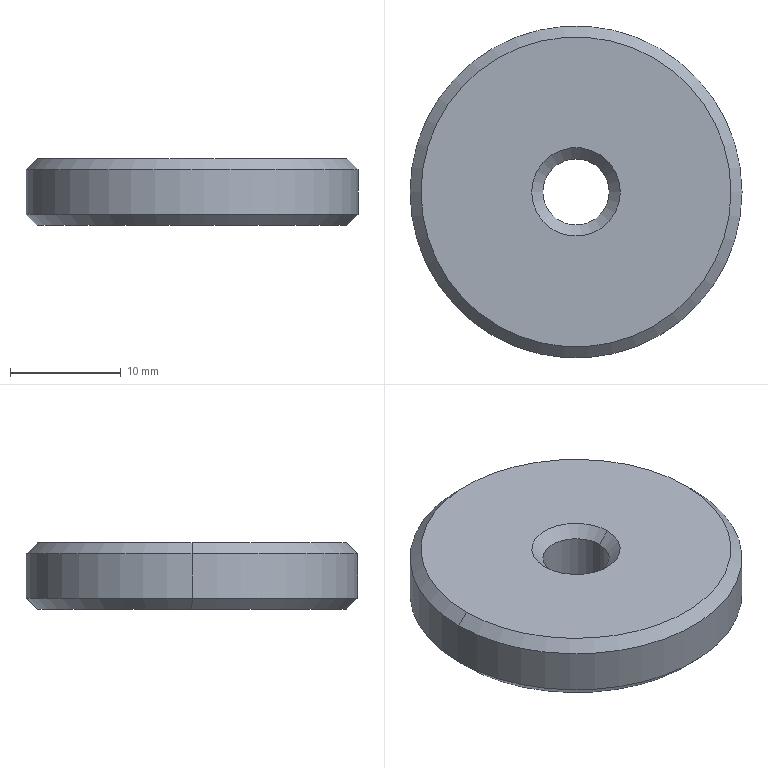Part | STEP file | Pressure plate | 1 solid | 14 faces | box 30 x 30 x 6 mm | volume 3958 mm3 | cone 8 | cylinder 4 | plane 2 | commonest cylinder face diameters 6 x2 30 x2
STEP:
#1=CARTESIAN_POINT('',(14.,0.,0.));
#2=VERTEX_POINT('',#1);
#3=CARTESIAN_POINT('',(-14.,0.,0.));
#4=VERTEX_POINT('',#3);
#5=CARTESIAN_POINT('',(0.,0.,0.));
#6=DIRECTION('',(0.,0.,1.));
#7=DIRECTION('',(1.,0.,0.));
#8=AXIS2_PLACEMENT_3D('',#5,#6,#7);
#9=CIRCLE('',#8,14.);
#10=EDGE_CURVE('',#2,#4,#9,.T.);
#11=ORIENTED_EDGE('',*,*,#10,.T.);
#12=CARTESIAN_POINT('',(-15.,0.,1.));
#13=VERTEX_POINT('',#12);
#14=CARTESIAN_POINT('',(-15.,0.,1.));
#15=DIRECTION('',(-0.7071,0.,0.7071));
#16=VECTOR('',#15,1000.);
#17=LINE('',#14,#16);
#18=EDGE_CURVE('',#4,#13,#17,.T.);
#19=ORIENTED_EDGE('',*,*,#18,.T.);
#20=CARTESIAN_POINT('',(15.,0.,1.));
#21=VERTEX_POINT('',#20);
#22=CARTESIAN_POINT('',(0.,0.,1.));
#23=DIRECTION('',(0.,0.,-1.));
#24=DIRECTION('',(1.,0.,0.));
#25=AXIS2_PLACEMENT_3D('',#22,#23,#24);
#26=CIRCLE('',#25,15.);
#27=EDGE_CURVE('',#13,#21,#26,.T.);
#28=ORIENTED_EDGE('',*,*,#27,.T.);
#29=CARTESIAN_POINT('',(15.,0.,1.));
#30=DIRECTION('',(0.7071,0.,0.7071));
#31=VECTOR('',#30,1000.);
#32=LINE('',#29,#31);
#33=EDGE_CURVE('',#2,#21,#32,.T.);
#34=ORIENTED_EDGE('',*,*,#33,.F.);
#35=EDGE_LOOP('',(#11,#19,#28,#34));
#36=FACE_OUTER_BOUND('',#35,.T.);
#37=CARTESIAN_POINT('',(0.,0.,1.));
#38=DIRECTION('',(0.,0.,1.));
#39=DIRECTION('',(1.,0.,0.));
#40=AXIS2_PLACEMENT_3D('',#37,#38,#39);
#41=CONICAL_SURFACE('',#40,15.,0.7854);
#42=ADVANCED_FACE('',(#36),#41,.T.);
#43=CARTESIAN_POINT('',(3.,0.,1.));
#44=VERTEX_POINT('',#43);
#45=CARTESIAN_POINT('',(-3.,0.,1.));
#46=VERTEX_POINT('',#45);
#47=CARTESIAN_POINT('',(0.,0.,1.));
#48=DIRECTION('',(0.,0.,-1.));
#49=DIRECTION('',(-1.,0.,0.));
#50=AXIS2_PLACEMENT_3D('',#47,#48,#49);
#51=CIRCLE('',#50,3.);
#52=EDGE_CURVE('',#44,#46,#51,.T.);
#53=ORIENTED_EDGE('',*,*,#52,.F.);
#54=CARTESIAN_POINT('',(4.,0.,0.));
#55=VERTEX_POINT('',#54);
#56=CARTESIAN_POINT('',(4.,0.,0.));
#57=DIRECTION('',(0.7071,0.,-0.7071));
#58=VECTOR('',#57,1000.);
#59=LINE('',#56,#58);
#60=EDGE_CURVE('',#44,#55,#59,.T.);
#61=ORIENTED_EDGE('',*,*,#60,.T.);
#62=CARTESIAN_POINT('',(-4.,0.,0.));
#63=VERTEX_POINT('',#62);
#64=CARTESIAN_POINT('',(0.,0.,0.));
#65=DIRECTION('',(0.,0.,-1.));
#66=DIRECTION('',(-1.,0.,0.));
#67=AXIS2_PLACEMENT_3D('',#64,#65,#66);
#68=CIRCLE('',#67,4.);
#69=EDGE_CURVE('',#55,#63,#68,.T.);
#70=ORIENTED_EDGE('',*,*,#69,.T.);
#71=CARTESIAN_POINT('',(-4.,0.,0.));
#72=DIRECTION('',(-0.7071,0.,-0.7071));
#73=VECTOR('',#72,1000.);
#74=LINE('',#71,#73);
#75=EDGE_CURVE('',#46,#63,#74,.T.);
#76=ORIENTED_EDGE('',*,*,#75,.F.);
#77=EDGE_LOOP('',(#53,#61,#70,#76));
#78=FACE_OUTER_BOUND('',#77,.T.);
#79=CARTESIAN_POINT('',(0.,0.,0.));
#80=DIRECTION('',(0.,0.,-1.));
#81=DIRECTION('',(-1.,0.,0.));
#82=AXIS2_PLACEMENT_3D('',#79,#80,#81);
#83=CONICAL_SURFACE('',#82,4.,0.7854);
#84=ADVANCED_FACE('',(#78),#83,.F.);
#85=CARTESIAN_POINT('',(-15.,0.,5.));
#86=VERTEX_POINT('',#85);
#87=CARTESIAN_POINT('',(15.,0.,5.));
#88=VERTEX_POINT('',#87);
#89=CARTESIAN_POINT('',(0.,0.,5.));
#90=DIRECTION('',(0.,0.,-1.));
#91=DIRECTION('',(-1.,0.,0.));
#92=AXIS2_PLACEMENT_3D('',#89,#90,#91);
#93=CIRCLE('',#92,15.);
#94=EDGE_CURVE('',#86,#88,#93,.T.);
#95=ORIENTED_EDGE('',*,*,#94,.T.);
#96=CARTESIAN_POINT('',(15.,0.,6.));
#97=DIRECTION('',(0.,0.,-1.));
#98=VECTOR('',#97,1000.);
#99=LINE('',#96,#98);
#100=EDGE_CURVE('',#88,#21,#99,.T.);
#101=ORIENTED_EDGE('',*,*,#100,.T.);
#102=ORIENTED_EDGE('',*,*,#27,.F.);
#103=CARTESIAN_POINT('',(-15.,0.,6.));
#104=DIRECTION('',(0.,0.,-1.));
#105=VECTOR('',#104,1000.);
#106=LINE('',#103,#105);
#107=EDGE_CURVE('',#86,#13,#106,.T.);
#108=ORIENTED_EDGE('',*,*,#107,.F.);
#109=EDGE_LOOP('',(#95,#101,#102,#108));
#110=FACE_OUTER_BOUND('',#109,.T.);
#111=CARTESIAN_POINT('',(0.,0.,6.));
#112=DIRECTION('',(0.,0.,-1.));
#113=DIRECTION('',(-1.,0.,0.));
#114=AXIS2_PLACEMENT_3D('',#111,#112,#113);
#115=CYLINDRICAL_SURFACE('',#114,15.);
#116=ADVANCED_FACE('',(#110),#115,.T.);
#117=CARTESIAN_POINT('',(3.,0.,5.));
#118=VERTEX_POINT('',#117);
#119=CARTESIAN_POINT('',(-3.,0.,5.));
#120=VERTEX_POINT('',#119);
#121=CARTESIAN_POINT('',(0.,0.,5.));
#122=DIRECTION('',(0.,0.,-1.));
#123=DIRECTION('',(-1.,0.,0.));
#124=AXIS2_PLACEMENT_3D('',#121,#122,#123);
#125=CIRCLE('',#124,3.);
#126=EDGE_CURVE('',#118,#120,#125,.T.);
#127=ORIENTED_EDGE('',*,*,#126,.F.);
#128=CARTESIAN_POINT('',(3.,0.,6.));
#129=DIRECTION('',(0.,0.,-1.));
#130=VECTOR('',#129,1000.);
#131=LINE('',#128,#130);
#132=EDGE_CURVE('',#118,#44,#131,.T.);
#133=ORIENTED_EDGE('',*,*,#132,.T.);
#134=ORIENTED_EDGE('',*,*,#52,.T.);
#135=CARTESIAN_POINT('',(-3.,0.,6.));
#136=DIRECTION('',(0.,0.,-1.));
#137=VECTOR('',#136,1000.);
#138=LINE('',#135,#137);
#139=EDGE_CURVE('',#120,#46,#138,.T.);
#140=ORIENTED_EDGE('',*,*,#139,.F.);
#141=EDGE_LOOP('',(#127,#133,#134,#140));
#142=FACE_OUTER_BOUND('',#141,.T.);
#143=CARTESIAN_POINT('',(0.,0.,6.));
#144=DIRECTION('',(0.,0.,-1.));
#145=DIRECTION('',(-1.,0.,0.));
#146=AXIS2_PLACEMENT_3D('',#143,#144,#145);
#147=CYLINDRICAL_SURFACE('',#146,3.);
#148=ADVANCED_FACE('',(#142),#147,.F.);
#149=CARTESIAN_POINT('',(-14.,0.,6.));
#150=VERTEX_POINT('',#149);
#151=CARTESIAN_POINT('',(14.,0.,6.));
#152=VERTEX_POINT('',#151);
#153=CARTESIAN_POINT('',(0.,0.,6.));
#154=DIRECTION('',(0.,0.,-1.));
#155=DIRECTION('',(-1.,0.,0.));
#156=AXIS2_PLACEMENT_3D('',#153,#154,#155);
#157=CIRCLE('',#156,14.);
#158=EDGE_CURVE('',#150,#152,#157,.T.);
#159=ORIENTED_EDGE('',*,*,#158,.T.);
#160=CARTESIAN_POINT('',(15.,0.,5.));
#161=DIRECTION('',(0.7071,0.,-0.7071));
#162=VECTOR('',#161,1000.);
#163=LINE('',#160,#162);
#164=EDGE_CURVE('',#152,#88,#163,.T.);
#165=ORIENTED_EDGE('',*,*,#164,.T.);
#166=ORIENTED_EDGE('',*,*,#94,.F.);
#167=CARTESIAN_POINT('',(-15.,0.,5.));
#168=DIRECTION('',(-0.7071,0.,-0.7071));
#169=VECTOR('',#168,1000.);
#170=LINE('',#167,#169);
#171=EDGE_CURVE('',#150,#86,#170,.T.);
#172=ORIENTED_EDGE('',*,*,#171,.F.);
#173=EDGE_LOOP('',(#159,#165,#166,#172));
#174=FACE_OUTER_BOUND('',#173,.T.);
#175=CARTESIAN_POINT('',(0.,0.,5.));
#176=DIRECTION('',(0.,0.,-1.));
#177=DIRECTION('',(-1.,0.,0.));
#178=AXIS2_PLACEMENT_3D('',#175,#176,#177);
#179=CONICAL_SURFACE('',#178,15.,0.7854);
#180=ADVANCED_FACE('',(#174),#179,.T.);
#181=ORIENTED_EDGE('',*,*,#126,.T.);
#182=CARTESIAN_POINT('',(-4.,0.,6.));
#183=VERTEX_POINT('',#182);
#184=CARTESIAN_POINT('',(-4.,0.,6.));
#185=DIRECTION('',(-0.7071,0.,0.7071));
#186=VECTOR('',#185,1000.);
#187=LINE('',#184,#186);
#188=EDGE_CURVE('',#120,#183,#187,.T.);
#189=ORIENTED_EDGE('',*,*,#188,.T.);
#190=CARTESIAN_POINT('',(4.,0.,6.));
#191=VERTEX_POINT('',#190);
#192=CARTESIAN_POINT('',(0.,0.,6.));
#193=DIRECTION('',(0.,0.,-1.));
#194=DIRECTION('',(1.,0.,0.));
#195=AXIS2_PLACEMENT_3D('',#192,#193,#194);
#196=CIRCLE('',#195,4.);
#197=EDGE_CURVE('',#191,#183,#196,.T.);
#198=ORIENTED_EDGE('',*,*,#197,.F.);
#199=CARTESIAN_POINT('',(4.,0.,6.));
#200=DIRECTION('',(0.7071,0.,0.7071));
#201=VECTOR('',#200,1000.);
#202=LINE('',#199,#201);
#203=EDGE_CURVE('',#118,#191,#202,.T.);
#204=ORIENTED_EDGE('',*,*,#203,.F.);
#205=EDGE_LOOP('',(#181,#189,#198,#204));
#206=FACE_OUTER_BOUND('',#205,.T.);
#207=CARTESIAN_POINT('',(0.,0.,6.));
#208=DIRECTION('',(0.,0.,1.));
#209=DIRECTION('',(1.,0.,0.));
#210=AXIS2_PLACEMENT_3D('',#207,#208,#209);
#211=CONICAL_SURFACE('',#210,4.,0.7854);
#212=ADVANCED_FACE('',(#206),#211,.F.);
#213=ORIENTED_EDGE('',*,*,#10,.F.);
#214=CARTESIAN_POINT('',(0.,0.,0.));
#215=DIRECTION('',(0.,0.,1.));
#216=DIRECTION('',(1.,0.,0.));
#217=AXIS2_PLACEMENT_3D('',#214,#215,#216);
#218=CIRCLE('',#217,14.);
#219=EDGE_CURVE('',#4,#2,#218,.T.);
#220=ORIENTED_EDGE('',*,*,#219,.F.);
#221=EDGE_LOOP('',(#213,#220));
#222=FACE_OUTER_BOUND('',#221,.T.);
#223=CARTESIAN_POINT('',(0.,0.,0.));
#224=DIRECTION('',(0.,0.,-1.));
#225=DIRECTION('',(-1.,0.,0.));
#226=AXIS2_PLACEMENT_3D('',#223,#224,#225);
#227=CIRCLE('',#226,4.);
#228=EDGE_CURVE('',#63,#55,#227,.T.);
#229=ORIENTED_EDGE('',*,*,#228,.F.);
#230=ORIENTED_EDGE('',*,*,#69,.F.);
#231=EDGE_LOOP('',(#229,#230));
#232=FACE_BOUND('',#231,.T.);
#233=CARTESIAN_POINT('',(0.,0.,0.));
#234=DIRECTION('',(0.,0.,1.));
#235=DIRECTION('',(1.,0.,0.));
#236=AXIS2_PLACEMENT_3D('',#233,#234,#235);
#237=PLANE('',#236);
#238=ADVANCED_FACE('',(#222,#232),#237,.F.);
#239=ORIENTED_EDGE('',*,*,#18,.F.);
#240=ORIENTED_EDGE('',*,*,#219,.T.);
#241=ORIENTED_EDGE('',*,*,#33,.T.);
#242=CARTESIAN_POINT('',(0.,0.,1.));
#243=DIRECTION('',(0.,0.,-1.));
#244=DIRECTION('',(1.,0.,0.));
#245=AXIS2_PLACEMENT_3D('',#242,#243,#244);
#246=CIRCLE('',#245,15.);
#247=EDGE_CURVE('',#21,#13,#246,.T.);
#248=ORIENTED_EDGE('',*,*,#247,.T.);
#249=EDGE_LOOP('',(#239,#240,#241,#248));
#250=FACE_OUTER_BOUND('',#249,.T.);
#251=CARTESIAN_POINT('',(0.,0.,1.));
#252=DIRECTION('',(0.,0.,1.));
#253=DIRECTION('',(1.,0.,0.));
#254=AXIS2_PLACEMENT_3D('',#251,#252,#253);
#255=CONICAL_SURFACE('',#254,15.,0.7854);
#256=ADVANCED_FACE('',(#250),#255,.T.);
#257=ORIENTED_EDGE('',*,*,#60,.F.);
#258=CARTESIAN_POINT('',(0.,0.,1.));
#259=DIRECTION('',(0.,0.,-1.));
#260=DIRECTION('',(-1.,0.,0.));
#261=AXIS2_PLACEMENT_3D('',#258,#259,#260);
#262=CIRCLE('',#261,3.);
#263=EDGE_CURVE('',#46,#44,#262,.T.);
#264=ORIENTED_EDGE('',*,*,#263,.F.);
#265=ORIENTED_EDGE('',*,*,#75,.T.);
#266=ORIENTED_EDGE('',*,*,#228,.T.);
#267=EDGE_LOOP('',(#257,#264,#265,#266));
#268=FACE_OUTER_BOUND('',#267,.T.);
#269=CARTESIAN_POINT('',(0.,0.,0.));
#270=DIRECTION('',(0.,0.,-1.));
#271=DIRECTION('',(-1.,0.,0.));
#272=AXIS2_PLACEMENT_3D('',#269,#270,#271);
#273=CONICAL_SURFACE('',#272,4.,0.7854);
#274=ADVANCED_FACE('',(#268),#273,.F.);
#275=ORIENTED_EDGE('',*,*,#100,.F.);
#276=CARTESIAN_POINT('',(0.,0.,5.));
#277=DIRECTION('',(0.,0.,-1.));
#278=DIRECTION('',(-1.,0.,0.));
#279=AXIS2_PLACEMENT_3D('',#276,#277,#278);
#280=CIRCLE('',#279,15.);
#281=EDGE_CURVE('',#88,#86,#280,.T.);
#282=ORIENTED_EDGE('',*,*,#281,.T.);
#283=ORIENTED_EDGE('',*,*,#107,.T.);
#284=ORIENTED_EDGE('',*,*,#247,.F.);
#285=EDGE_LOOP('',(#275,#282,#283,#284));
#286=FACE_OUTER_BOUND('',#285,.T.);
#287=CARTESIAN_POINT('',(0.,0.,6.));
#288=DIRECTION('',(0.,0.,-1.));
#289=DIRECTION('',(-1.,0.,0.));
#290=AXIS2_PLACEMENT_3D('',#287,#288,#289);
#291=CYLINDRICAL_SURFACE('',#290,15.);
#292=ADVANCED_FACE('',(#286),#291,.T.);
#293=ORIENTED_EDGE('',*,*,#132,.F.);
#294=CARTESIAN_POINT('',(0.,0.,5.));
#295=DIRECTION('',(0.,0.,-1.));
#296=DIRECTION('',(-1.,0.,0.));
#297=AXIS2_PLACEMENT_3D('',#294,#295,#296);
#298=CIRCLE('',#297,3.);
#299=EDGE_CURVE('',#120,#118,#298,.T.);
#300=ORIENTED_EDGE('',*,*,#299,.F.);
#301=ORIENTED_EDGE('',*,*,#139,.T.);
#302=ORIENTED_EDGE('',*,*,#263,.T.);
#303=EDGE_LOOP('',(#293,#300,#301,#302));
#304=FACE_OUTER_BOUND('',#303,.T.);
#305=CARTESIAN_POINT('',(0.,0.,6.));
#306=DIRECTION('',(0.,0.,-1.));
#307=DIRECTION('',(-1.,0.,0.));
#308=AXIS2_PLACEMENT_3D('',#305,#306,#307);
#309=CYLINDRICAL_SURFACE('',#308,3.);
#310=ADVANCED_FACE('',(#304),#309,.F.);
#311=ORIENTED_EDGE('',*,*,#164,.F.);
#312=CARTESIAN_POINT('',(0.,0.,6.));
#313=DIRECTION('',(0.,0.,-1.));
#314=DIRECTION('',(-1.,0.,0.));
#315=AXIS2_PLACEMENT_3D('',#312,#313,#314);
#316=CIRCLE('',#315,14.);
#317=EDGE_CURVE('',#152,#150,#316,.T.);
#318=ORIENTED_EDGE('',*,*,#317,.T.);
#319=ORIENTED_EDGE('',*,*,#171,.T.);
#320=ORIENTED_EDGE('',*,*,#281,.F.);
#321=EDGE_LOOP('',(#311,#318,#319,#320));
#322=FACE_OUTER_BOUND('',#321,.T.);
#323=CARTESIAN_POINT('',(0.,0.,5.));
#324=DIRECTION('',(0.,0.,-1.));
#325=DIRECTION('',(-1.,0.,0.));
#326=AXIS2_PLACEMENT_3D('',#323,#324,#325);
#327=CONICAL_SURFACE('',#326,15.,0.7854);
#328=ADVANCED_FACE('',(#322),#327,.T.);
#329=ORIENTED_EDGE('',*,*,#188,.F.);
#330=ORIENTED_EDGE('',*,*,#299,.T.);
#331=ORIENTED_EDGE('',*,*,#203,.T.);
#332=CARTESIAN_POINT('',(0.,0.,6.));
#333=DIRECTION('',(0.,0.,-1.));
#334=DIRECTION('',(1.,0.,0.));
#335=AXIS2_PLACEMENT_3D('',#332,#333,#334);
#336=CIRCLE('',#335,4.);
#337=EDGE_CURVE('',#183,#191,#336,.T.);
#338=ORIENTED_EDGE('',*,*,#337,.F.);
#339=EDGE_LOOP('',(#329,#330,#331,#338));
#340=FACE_OUTER_BOUND('',#339,.T.);
#341=CARTESIAN_POINT('',(0.,0.,6.));
#342=DIRECTION('',(0.,0.,1.));
#343=DIRECTION('',(1.,0.,0.));
#344=AXIS2_PLACEMENT_3D('',#341,#342,#343);
#345=CONICAL_SURFACE('',#344,4.,0.7854);
#346=ADVANCED_FACE('',(#340),#345,.F.);
#347=ORIENTED_EDGE('',*,*,#158,.F.);
#348=ORIENTED_EDGE('',*,*,#317,.F.);
#349=EDGE_LOOP('',(#347,#348));
#350=FACE_OUTER_BOUND('',#349,.T.);
#351=ORIENTED_EDGE('',*,*,#197,.T.);
#352=ORIENTED_EDGE('',*,*,#337,.T.);
#353=EDGE_LOOP('',(#351,#352));
#354=FACE_BOUND('',#353,.T.);
#355=CARTESIAN_POINT('',(0.,0.,6.));
#356=DIRECTION('',(0.,0.,1.));
#357=DIRECTION('',(1.,0.,0.));
#358=AXIS2_PLACEMENT_3D('',#355,#356,#357);
#359=PLANE('',#358);
#360=ADVANCED_FACE('',(#350,#354),#359,.T.);
#361=CLOSED_SHELL('',(#42,#84,#116,#148,#180,#212,#238,#256,#274,#292,#310,#328,#346,#360));
#362=MANIFOLD_SOLID_BREP('',#361);
#363=CARTESIAN_POINT('',(0.,0.,0.));
#364=DIRECTION('',(0.,0.,1.));
#365=DIRECTION('',(1.,0.,0.));
#366=AXIS2_PLACEMENT_3D('',#363,#364,#365);
#367=(LENGTH_UNIT()NAMED_UNIT(*)SI_UNIT(.MILLI.,.METRE.));
#368=UNCERTAINTY_MEASURE_WITH_UNIT(LENGTH_MEASURE(0.00001),#367,'','');
#369=(NAMED_UNIT(*)PLANE_ANGLE_UNIT()SI_UNIT($,.RADIAN.));
#370=(NAMED_UNIT(*)SI_UNIT($,.STERADIAN.)SOLID_ANGLE_UNIT());
#371=(GEOMETRIC_REPRESENTATION_CONTEXT(3)GLOBAL_UNCERTAINTY_ASSIGNED_CONTEXT((#368))GLOBAL_UNIT_ASSIGNED_CONTEXT((#367,#369,#370))REPRESENTATION_CONTEXT('',''));
#372=ADVANCED_BREP_SHAPE_REPRESENTATION('',(#362,#366),#371);